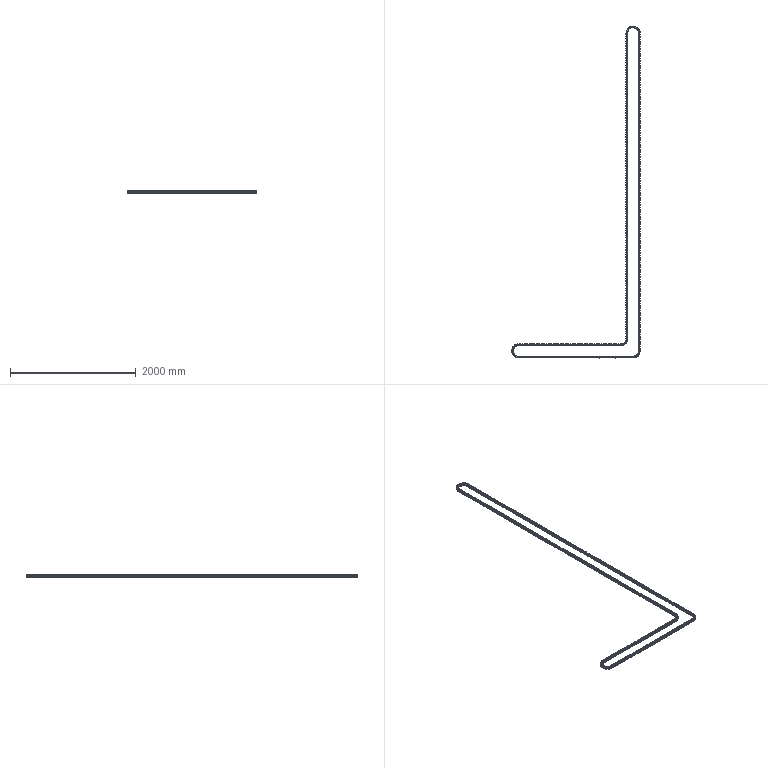Part | STEP file | Inner chain 1XG | 187 solids | 4114 faces | volume 4855051 mm3 | cylinder 3366 | plane 748 | commonest cylinder face diameters 30 x1122 8 x748 18 x748 64.25 x748